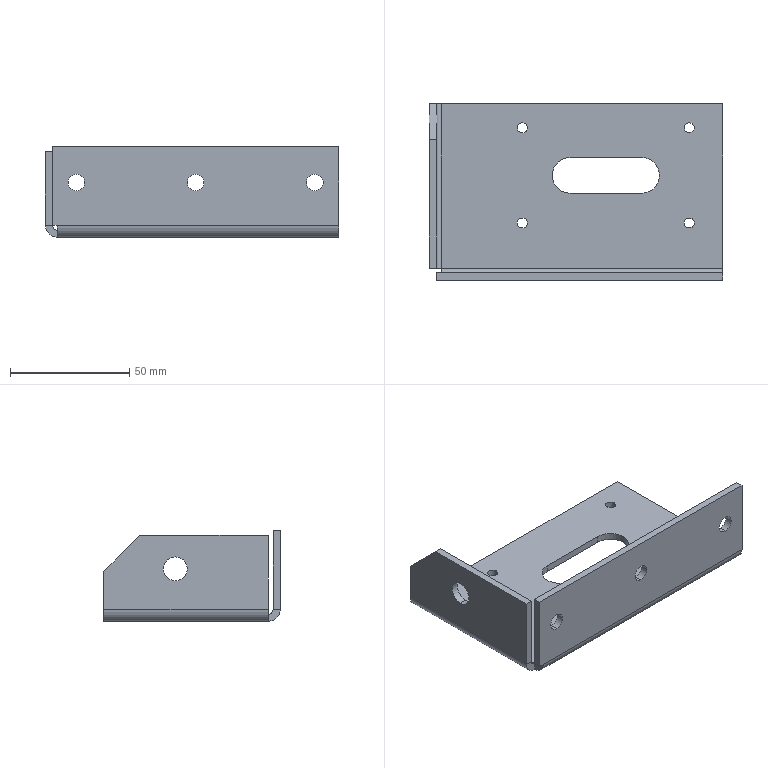Part | NX | features BREP 1 | 1 solid | 45 faces | box 123 x 74 x 38 mm | volume 42841 mm3 | cylinder 23 | plane 22 | commonest cylinder face diameters 4.2 x8 7 x6 10 x4 15 x3 4 x2
STEP:
#1=CARTESIAN_POINT('',(-123.,59.,-2.));
#2=VERTEX_POINT('',#1);
#3=CARTESIAN_POINT('',(-123.,74.,-17.));
#4=VERTEX_POINT('',#3);
#5=CARTESIAN_POINT('',(-123.,28.5,28.5));
#6=DIRECTION('',(0.,0.7071,-0.7071));
#7=VECTOR('',#6,1000.);
#8=LINE('',#5,#7);
#9=EDGE_CURVE('',#2,#4,#8,.T.);
#10=ORIENTED_EDGE('',*,*,#9,.F.);
#11=CARTESIAN_POINT('',(-120.,59.,-2.));
#12=VERTEX_POINT('',#11);
#13=CARTESIAN_POINT('',(-123.,59.,-2.));
#14=DIRECTION('',(-1.,0.,0.));
#15=VECTOR('',#14,1000.);
#16=LINE('',#13,#15);
#17=EDGE_CURVE('',#12,#2,#16,.T.);
#18=ORIENTED_EDGE('',*,*,#17,.F.);
#19=CARTESIAN_POINT('',(-120.,74.,-17.));
#20=VERTEX_POINT('',#19);
#21=CARTESIAN_POINT('',(-120.,74.,-17.));
#22=DIRECTION('',(0.,-0.7071,0.7071));
#23=VECTOR('',#22,1000.);
#24=LINE('',#21,#23);
#25=EDGE_CURVE('',#20,#12,#24,.T.);
#26=ORIENTED_EDGE('',*,*,#25,.F.);
#27=CARTESIAN_POINT('',(-123.,74.,-17.));
#28=DIRECTION('',(1.,0.,0.));
#29=VECTOR('',#28,1000.);
#30=LINE('',#27,#29);
#31=EDGE_CURVE('',#4,#20,#30,.T.);
#32=ORIENTED_EDGE('',*,*,#31,.F.);
#33=EDGE_LOOP('',(#10,#18,#26,#32));
#34=FACE_BOUND('',#33,.T.);
#35=CARTESIAN_POINT('',(-123.,74.,-17.));
#36=DIRECTION('',(0.,-0.7071,-0.7071));
#37=DIRECTION('',(1.,0.,0.));
#38=AXIS2_PLACEMENT_3D('',#35,#36,#37);
#39=PLANE('',#38);
#40=ADVANCED_FACE('',(#34),#39,.F.);
#41=CARTESIAN_POINT('',(-110.,3.,-18.5));
#42=VERTEX_POINT('',#41);
#43=CARTESIAN_POINT('',(-110.,0.,-18.5));
#44=VERTEX_POINT('',#43);
#45=CARTESIAN_POINT('',(-110.,3.,-18.5));
#46=DIRECTION('',(0.,1.,0.));
#47=VECTOR('',#46,1000.);
#48=LINE('',#45,#47);
#49=EDGE_CURVE('',#42,#44,#48,.F.);
#50=ORIENTED_EDGE('',*,*,#49,.T.);
#51=CARTESIAN_POINT('',(-110.,0.,-11.5));
#52=VERTEX_POINT('',#51);
#53=CARTESIAN_POINT('',(-110.,0.,-15.));
#54=DIRECTION('',(0.,1.,0.));
#55=DIRECTION('',(0.,0.,1.));
#56=AXIS2_PLACEMENT_3D('',#53,#54,#55);
#57=CIRCLE('',#56,3.5);
#58=EDGE_CURVE('',#52,#44,#57,.T.);
#59=ORIENTED_EDGE('',*,*,#58,.F.);
#60=CARTESIAN_POINT('',(-110.,3.,-11.5));
#61=VERTEX_POINT('',#60);
#62=CARTESIAN_POINT('',(-110.,3.,-11.5));
#63=DIRECTION('',(0.,1.,0.));
#64=VECTOR('',#63,1000.);
#65=LINE('',#62,#64);
#66=EDGE_CURVE('',#61,#52,#65,.F.);
#67=ORIENTED_EDGE('',*,*,#66,.F.);
#68=CARTESIAN_POINT('',(-110.,3.,-15.));
#69=DIRECTION('',(0.,1.,0.));
#70=DIRECTION('',(0.,0.,1.));
#71=AXIS2_PLACEMENT_3D('',#68,#69,#70);
#72=CIRCLE('',#71,3.5);
#73=EDGE_CURVE('',#61,#42,#72,.T.);
#74=ORIENTED_EDGE('',*,*,#73,.T.);
#75=EDGE_LOOP('',(#50,#59,#67,#74));
#76=FACE_BOUND('',#75,.T.);
#77=CARTESIAN_POINT('',(-110.,3.,-15.));
#78=DIRECTION('',(0.,1.,0.));
#79=DIRECTION('',(0.,0.,1.));
#80=AXIS2_PLACEMENT_3D('',#77,#78,#79);
#81=CYLINDRICAL_SURFACE('',#80,3.5);
#82=ADVANCED_FACE('',(#76),#81,.F.);
#83=CARTESIAN_POINT('',(-60.,3.,-18.5));
#84=VERTEX_POINT('',#83);
#85=CARTESIAN_POINT('',(-60.,0.,-18.5));
#86=VERTEX_POINT('',#85);
#87=CARTESIAN_POINT('',(-60.,3.,-18.5));
#88=DIRECTION('',(0.,1.,0.));
#89=VECTOR('',#88,1000.);
#90=LINE('',#87,#89);
#91=EDGE_CURVE('',#84,#86,#90,.F.);
#92=ORIENTED_EDGE('',*,*,#91,.T.);
#93=CARTESIAN_POINT('',(-60.,0.,-11.5));
#94=VERTEX_POINT('',#93);
#95=CARTESIAN_POINT('',(-60.,0.,-15.));
#96=DIRECTION('',(0.,1.,0.));
#97=DIRECTION('',(0.,0.,1.));
#98=AXIS2_PLACEMENT_3D('',#95,#96,#97);
#99=CIRCLE('',#98,3.5);
#100=EDGE_CURVE('',#94,#86,#99,.T.);
#101=ORIENTED_EDGE('',*,*,#100,.F.);
#102=CARTESIAN_POINT('',(-60.,3.,-11.5));
#103=VERTEX_POINT('',#102);
#104=CARTESIAN_POINT('',(-60.,3.,-11.5));
#105=DIRECTION('',(0.,1.,0.));
#106=VECTOR('',#105,1000.);
#107=LINE('',#104,#106);
#108=EDGE_CURVE('',#103,#94,#107,.F.);
#109=ORIENTED_EDGE('',*,*,#108,.F.);
#110=CARTESIAN_POINT('',(-60.,3.,-15.));
#111=DIRECTION('',(0.,1.,0.));
#112=DIRECTION('',(0.,0.,1.));
#113=AXIS2_PLACEMENT_3D('',#110,#111,#112);
#114=CIRCLE('',#113,3.5);
#115=EDGE_CURVE('',#103,#84,#114,.T.);
#116=ORIENTED_EDGE('',*,*,#115,.T.);
#117=EDGE_LOOP('',(#92,#101,#109,#116));
#118=FACE_BOUND('',#117,.T.);
#119=CARTESIAN_POINT('',(-60.,3.,-15.));
#120=DIRECTION('',(0.,1.,0.));
#121=DIRECTION('',(0.,0.,1.));
#122=AXIS2_PLACEMENT_3D('',#119,#120,#121);
#123=CYLINDRICAL_SURFACE('',#122,3.5);
#124=ADVANCED_FACE('',(#118),#123,.F.);
#125=CARTESIAN_POINT('',(-10.,3.,-18.5));
#126=VERTEX_POINT('',#125);
#127=CARTESIAN_POINT('',(-10.,0.,-18.5));
#128=VERTEX_POINT('',#127);
#129=CARTESIAN_POINT('',(-10.,3.,-18.5));
#130=DIRECTION('',(0.,1.,0.));
#131=VECTOR('',#130,1000.);
#132=LINE('',#129,#131);
#133=EDGE_CURVE('',#126,#128,#132,.F.);
#134=ORIENTED_EDGE('',*,*,#133,.T.);
#135=CARTESIAN_POINT('',(-10.,0.,-11.5));
#136=VERTEX_POINT('',#135);
#137=CARTESIAN_POINT('',(-10.,0.,-15.));
#138=DIRECTION('',(0.,1.,0.));
#139=DIRECTION('',(0.,0.,1.));
#140=AXIS2_PLACEMENT_3D('',#137,#138,#139);
#141=CIRCLE('',#140,3.5);
#142=EDGE_CURVE('',#136,#128,#141,.T.);
#143=ORIENTED_EDGE('',*,*,#142,.F.);
#144=CARTESIAN_POINT('',(-10.,3.,-11.5));
#145=VERTEX_POINT('',#144);
#146=CARTESIAN_POINT('',(-10.,3.,-11.5));
#147=DIRECTION('',(0.,1.,0.));
#148=VECTOR('',#147,1000.);
#149=LINE('',#146,#148);
#150=EDGE_CURVE('',#145,#136,#149,.F.);
#151=ORIENTED_EDGE('',*,*,#150,.F.);
#152=CARTESIAN_POINT('',(-10.,3.,-15.));
#153=DIRECTION('',(0.,1.,0.));
#154=DIRECTION('',(0.,0.,1.));
#155=AXIS2_PLACEMENT_3D('',#152,#153,#154);
#156=CIRCLE('',#155,3.5);
#157=EDGE_CURVE('',#145,#126,#156,.T.);
#158=ORIENTED_EDGE('',*,*,#157,.T.);
#159=EDGE_LOOP('',(#134,#143,#151,#158));
#160=FACE_BOUND('',#159,.T.);
#161=CARTESIAN_POINT('',(-10.,3.,-15.));
#162=DIRECTION('',(0.,1.,0.));
#163=DIRECTION('',(0.,0.,1.));
#164=AXIS2_PLACEMENT_3D('',#161,#162,#163);
#165=CYLINDRICAL_SURFACE('',#164,3.5);
#166=ADVANCED_FACE('',(#160),#165,.F.);
#167=CARTESIAN_POINT('',(-86.1,64.,-35.));
#168=VERTEX_POINT('',#167);
#169=CARTESIAN_POINT('',(-86.1,64.,-38.));
#170=VERTEX_POINT('',#169);
#171=CARTESIAN_POINT('',(-86.1,64.,-35.));
#172=DIRECTION('',(0.,0.,1.));
#173=VECTOR('',#172,1000.);
#174=LINE('',#171,#173);
#175=EDGE_CURVE('',#168,#170,#174,.F.);
#176=ORIENTED_EDGE('',*,*,#175,.T.);
#177=CARTESIAN_POINT('',(-81.9,64.,-38.));
#178=VERTEX_POINT('',#177);
#179=CARTESIAN_POINT('',(-84.,64.,-38.));
#180=DIRECTION('',(0.,0.,1.));
#181=DIRECTION('',(1.,0.,0.));
#182=AXIS2_PLACEMENT_3D('',#179,#180,#181);
#183=CIRCLE('',#182,2.1);
#184=EDGE_CURVE('',#178,#170,#183,.T.);
#185=ORIENTED_EDGE('',*,*,#184,.F.);
#186=CARTESIAN_POINT('',(-81.9,64.,-35.));
#187=VERTEX_POINT('',#186);
#188=CARTESIAN_POINT('',(-81.9,64.,-35.));
#189=DIRECTION('',(0.,0.,1.));
#190=VECTOR('',#189,1000.);
#191=LINE('',#188,#190);
#192=EDGE_CURVE('',#187,#178,#191,.F.);
#193=ORIENTED_EDGE('',*,*,#192,.F.);
#194=CARTESIAN_POINT('',(-84.,64.,-35.));
#195=DIRECTION('',(0.,0.,1.));
#196=DIRECTION('',(1.,0.,0.));
#197=AXIS2_PLACEMENT_3D('',#194,#195,#196);
#198=CIRCLE('',#197,2.1);
#199=EDGE_CURVE('',#187,#168,#198,.T.);
#200=ORIENTED_EDGE('',*,*,#199,.T.);
#201=EDGE_LOOP('',(#176,#185,#193,#200));
#202=FACE_BOUND('',#201,.T.);
#203=CARTESIAN_POINT('',(-84.,64.,-35.));
#204=DIRECTION('',(0.,0.,1.));
#205=DIRECTION('',(1.,0.,0.));
#206=AXIS2_PLACEMENT_3D('',#203,#204,#205);
#207=CYLINDRICAL_SURFACE('',#206,2.1);
#208=ADVANCED_FACE('',(#202),#207,.F.);
#209=CARTESIAN_POINT('',(-86.1,24.,-35.));
#210=VERTEX_POINT('',#209);
#211=CARTESIAN_POINT('',(-86.1,24.,-38.));
#212=VERTEX_POINT('',#211);
#213=CARTESIAN_POINT('',(-86.1,24.,-35.));
#214=DIRECTION('',(0.,0.,1.));
#215=VECTOR('',#214,1000.);
#216=LINE('',#213,#215);
#217=EDGE_CURVE('',#210,#212,#216,.F.);
#218=ORIENTED_EDGE('',*,*,#217,.T.);
#219=CARTESIAN_POINT('',(-81.9,24.,-38.));
#220=VERTEX_POINT('',#219);
#221=CARTESIAN_POINT('',(-84.,24.,-38.));
#222=DIRECTION('',(0.,0.,1.));
#223=DIRECTION('',(1.,0.,0.));
#224=AXIS2_PLACEMENT_3D('',#221,#222,#223);
#225=CIRCLE('',#224,2.1);
#226=EDGE_CURVE('',#220,#212,#225,.T.);
#227=ORIENTED_EDGE('',*,*,#226,.F.);
#228=CARTESIAN_POINT('',(-81.9,24.,-35.));
#229=VERTEX_POINT('',#228);
#230=CARTESIAN_POINT('',(-81.9,24.,-35.));
#231=DIRECTION('',(0.,0.,1.));
#232=VECTOR('',#231,1000.);
#233=LINE('',#230,#232);
#234=EDGE_CURVE('',#229,#220,#233,.F.);
#235=ORIENTED_EDGE('',*,*,#234,.F.);
#236=CARTESIAN_POINT('',(-84.,24.,-35.));
#237=DIRECTION('',(0.,0.,1.));
#238=DIRECTION('',(1.,0.,0.));
#239=AXIS2_PLACEMENT_3D('',#236,#237,#238);
#240=CIRCLE('',#239,2.1);
#241=EDGE_CURVE('',#229,#210,#240,.T.);
#242=ORIENTED_EDGE('',*,*,#241,.T.);
#243=EDGE_LOOP('',(#218,#227,#235,#242));
#244=FACE_BOUND('',#243,.T.);
#245=CARTESIAN_POINT('',(-84.,24.,-35.));
#246=DIRECTION('',(0.,0.,1.));
#247=DIRECTION('',(1.,0.,0.));
#248=AXIS2_PLACEMENT_3D('',#245,#246,#247);
#249=CYLINDRICAL_SURFACE('',#248,2.1);
#250=ADVANCED_FACE('',(#244),#249,.F.);
#251=CARTESIAN_POINT('',(-16.1,24.,-35.));
#252=VERTEX_POINT('',#251);
#253=CARTESIAN_POINT('',(-16.1,24.,-38.));
#254=VERTEX_POINT('',#253);
#255=CARTESIAN_POINT('',(-16.1,24.,-35.));
#256=DIRECTION('',(0.,0.,1.));
#257=VECTOR('',#256,1000.);
#258=LINE('',#255,#257);
#259=EDGE_CURVE('',#252,#254,#258,.F.);
#260=ORIENTED_EDGE('',*,*,#259,.T.);
#261=CARTESIAN_POINT('',(-11.9,24.,-38.));
#262=VERTEX_POINT('',#261);
#263=CARTESIAN_POINT('',(-14.,24.,-38.));
#264=DIRECTION('',(0.,0.,1.));
#265=DIRECTION('',(1.,0.,0.));
#266=AXIS2_PLACEMENT_3D('',#263,#264,#265);
#267=CIRCLE('',#266,2.1);
#268=EDGE_CURVE('',#262,#254,#267,.T.);
#269=ORIENTED_EDGE('',*,*,#268,.F.);
#270=CARTESIAN_POINT('',(-11.9,24.,-35.));
#271=VERTEX_POINT('',#270);
#272=CARTESIAN_POINT('',(-11.9,24.,-35.));
#273=DIRECTION('',(0.,0.,1.));
#274=VECTOR('',#273,1000.);
#275=LINE('',#272,#274);
#276=EDGE_CURVE('',#271,#262,#275,.F.);
#277=ORIENTED_EDGE('',*,*,#276,.F.);
#278=CARTESIAN_POINT('',(-14.,24.,-35.));
#279=DIRECTION('',(0.,0.,1.));
#280=DIRECTION('',(1.,0.,0.));
#281=AXIS2_PLACEMENT_3D('',#278,#279,#280);
#282=CIRCLE('',#281,2.1);
#283=EDGE_CURVE('',#271,#252,#282,.T.);
#284=ORIENTED_EDGE('',*,*,#283,.T.);
#285=EDGE_LOOP('',(#260,#269,#277,#284));
#286=FACE_BOUND('',#285,.T.);
#287=CARTESIAN_POINT('',(-14.,24.,-35.));
#288=DIRECTION('',(0.,0.,1.));
#289=DIRECTION('',(1.,0.,0.));
#290=AXIS2_PLACEMENT_3D('',#287,#288,#289);
#291=CYLINDRICAL_SURFACE('',#290,2.1);
#292=ADVANCED_FACE('',(#286),#291,.F.);
#293=CARTESIAN_POINT('',(-16.1,64.,-35.));
#294=VERTEX_POINT('',#293);
#295=CARTESIAN_POINT('',(-16.1,64.,-38.));
#296=VERTEX_POINT('',#295);
#297=CARTESIAN_POINT('',(-16.1,64.,-35.));
#298=DIRECTION('',(0.,0.,1.));
#299=VECTOR('',#298,1000.);
#300=LINE('',#297,#299);
#301=EDGE_CURVE('',#294,#296,#300,.F.);
#302=ORIENTED_EDGE('',*,*,#301,.T.);
#303=CARTESIAN_POINT('',(-11.9,64.,-38.));
#304=VERTEX_POINT('',#303);
#305=CARTESIAN_POINT('',(-14.,64.,-38.));
#306=DIRECTION('',(0.,0.,1.));
#307=DIRECTION('',(1.,0.,0.));
#308=AXIS2_PLACEMENT_3D('',#305,#306,#307);
#309=CIRCLE('',#308,2.1);
#310=EDGE_CURVE('',#304,#296,#309,.T.);
#311=ORIENTED_EDGE('',*,*,#310,.F.);
#312=CARTESIAN_POINT('',(-11.9,64.,-35.));
#313=VERTEX_POINT('',#312);
#314=CARTESIAN_POINT('',(-11.9,64.,-35.));
#315=DIRECTION('',(0.,0.,1.));
#316=VECTOR('',#315,1000.);
#317=LINE('',#314,#316);
#318=EDGE_CURVE('',#313,#304,#317,.F.);
#319=ORIENTED_EDGE('',*,*,#318,.F.);
#320=CARTESIAN_POINT('',(-14.,64.,-35.));
#321=DIRECTION('',(0.,0.,1.));
#322=DIRECTION('',(1.,0.,0.));
#323=AXIS2_PLACEMENT_3D('',#320,#321,#322);
#324=CIRCLE('',#323,2.1);
#325=EDGE_CURVE('',#313,#294,#324,.T.);
#326=ORIENTED_EDGE('',*,*,#325,.T.);
#327=EDGE_LOOP('',(#302,#311,#319,#326));
#328=FACE_BOUND('',#327,.T.);
#329=CARTESIAN_POINT('',(-14.,64.,-35.));
#330=DIRECTION('',(0.,0.,1.));
#331=DIRECTION('',(1.,0.,0.));
#332=AXIS2_PLACEMENT_3D('',#329,#330,#331);
#333=CYLINDRICAL_SURFACE('',#332,2.1);
#334=ADVANCED_FACE('',(#328),#333,.F.);
#335=CARTESIAN_POINT('',(-34.,51.5,-35.));
#336=VERTEX_POINT('',#335);
#337=CARTESIAN_POINT('',(-64.,51.5,-35.));
#338=VERTEX_POINT('',#337);
#339=CARTESIAN_POINT('',(-34.,51.5,-35.));
#340=DIRECTION('',(-1.,0.,0.));
#341=VECTOR('',#340,1000.);
#342=LINE('',#339,#341);
#343=EDGE_CURVE('',#336,#338,#342,.T.);
#344=ORIENTED_EDGE('',*,*,#343,.T.);
#345=CARTESIAN_POINT('',(-64.,51.5,-38.));
#346=VERTEX_POINT('',#345);
#347=CARTESIAN_POINT('',(-64.,51.5,-38.));
#348=DIRECTION('',(0.,0.,1.));
#349=VECTOR('',#348,1000.);
#350=LINE('',#347,#349);
#351=EDGE_CURVE('',#346,#338,#350,.T.);
#352=ORIENTED_EDGE('',*,*,#351,.F.);
#353=CARTESIAN_POINT('',(-34.,51.5,-38.));
#354=VERTEX_POINT('',#353);
#355=CARTESIAN_POINT('',(-34.,51.5,-38.));
#356=DIRECTION('',(-1.,0.,0.));
#357=VECTOR('',#356,1000.);
#358=LINE('',#355,#357);
#359=EDGE_CURVE('',#354,#346,#358,.T.);
#360=ORIENTED_EDGE('',*,*,#359,.F.);
#361=CARTESIAN_POINT('',(-34.,51.5,-38.));
#362=DIRECTION('',(0.,0.,1.));
#363=VECTOR('',#362,1000.);
#364=LINE('',#361,#363);
#365=EDGE_CURVE('',#354,#336,#364,.T.);
#366=ORIENTED_EDGE('',*,*,#365,.T.);
#367=EDGE_LOOP('',(#344,#352,#360,#366));
#368=FACE_BOUND('',#367,.T.);
#369=CARTESIAN_POINT('',(-34.,51.5,-38.));
#370=DIRECTION('',(0.,1.,0.));
#371=DIRECTION('',(0.,0.,1.));
#372=AXIS2_PLACEMENT_3D('',#369,#370,#371);
#373=PLANE('',#372);
#374=ADVANCED_FACE('',(#368),#373,.F.);
#375=CARTESIAN_POINT('',(-64.,36.5,-35.));
#376=VERTEX_POINT('',#375);
#377=CARTESIAN_POINT('',(-64.,44.,-35.));
#378=DIRECTION('',(0.,0.,1.));
#379=DIRECTION('',(1.,0.,0.));
#380=AXIS2_PLACEMENT_3D('',#377,#378,#379);
#381=CIRCLE('',#380,7.5);
#382=EDGE_CURVE('',#338,#376,#381,.T.);
#383=ORIENTED_EDGE('',*,*,#382,.T.);
#384=CARTESIAN_POINT('',(-64.,36.5,-38.));
#385=VERTEX_POINT('',#384);
#386=CARTESIAN_POINT('',(-64.,36.5,-38.));
#387=DIRECTION('',(0.,0.,1.));
#388=VECTOR('',#387,1000.);
#389=LINE('',#386,#388);
#390=EDGE_CURVE('',#385,#376,#389,.T.);
#391=ORIENTED_EDGE('',*,*,#390,.F.);
#392=CARTESIAN_POINT('',(-64.,44.,-38.));
#393=DIRECTION('',(0.,0.,1.));
#394=DIRECTION('',(1.,0.,0.));
#395=AXIS2_PLACEMENT_3D('',#392,#393,#394);
#396=CIRCLE('',#395,7.5);
#397=EDGE_CURVE('',#346,#385,#396,.T.);
#398=ORIENTED_EDGE('',*,*,#397,.F.);
#399=ORIENTED_EDGE('',*,*,#351,.T.);
#400=EDGE_LOOP('',(#383,#391,#398,#399));
#401=FACE_BOUND('',#400,.T.);
#402=CARTESIAN_POINT('',(-64.,44.,-38.));
#403=DIRECTION('',(0.,0.,1.));
#404=DIRECTION('',(1.,0.,0.));
#405=AXIS2_PLACEMENT_3D('',#402,#403,#404);
#406=CYLINDRICAL_SURFACE('',#405,7.5);
#407=ADVANCED_FACE('',(#401),#406,.F.);
#408=CARTESIAN_POINT('',(-34.,36.5,-35.));
#409=VERTEX_POINT('',#408);
#410=CARTESIAN_POINT('',(-34.,36.5,-35.));
#411=DIRECTION('',(1.,0.,0.));
#412=VECTOR('',#411,1000.);
#413=LINE('',#410,#412);
#414=EDGE_CURVE('',#376,#409,#413,.T.);
#415=ORIENTED_EDGE('',*,*,#414,.T.);
#416=CARTESIAN_POINT('',(-34.,36.5,-38.));
#417=VERTEX_POINT('',#416);
#418=CARTESIAN_POINT('',(-34.,36.5,-38.));
#419=DIRECTION('',(0.,0.,1.));
#420=VECTOR('',#419,1000.);
#421=LINE('',#418,#420);
#422=EDGE_CURVE('',#417,#409,#421,.T.);
#423=ORIENTED_EDGE('',*,*,#422,.F.);
#424=CARTESIAN_POINT('',(-34.,36.5,-38.));
#425=DIRECTION('',(1.,0.,0.));
#426=VECTOR('',#425,1000.);
#427=LINE('',#424,#426);
#428=EDGE_CURVE('',#385,#417,#427,.T.);
#429=ORIENTED_EDGE('',*,*,#428,.F.);
#430=ORIENTED_EDGE('',*,*,#390,.T.);
#431=EDGE_LOOP('',(#415,#423,#429,#430));
#432=FACE_BOUND('',#431,.T.);
#433=CARTESIAN_POINT('',(-34.,36.5,-38.));
#434=DIRECTION('',(0.,-1.,0.));
#435=DIRECTION('',(1.,0.,0.));
#436=AXIS2_PLACEMENT_3D('',#433,#434,#435);
#437=PLANE('',#436);
#438=ADVANCED_FACE('',(#432),#437,.F.);
#439=CARTESIAN_POINT('',(-26.5,44.,-38.));
#440=VERTEX_POINT('',#439);
#441=CARTESIAN_POINT('',(-26.5,44.,-35.));
#442=VERTEX_POINT('',#441);
#443=CARTESIAN_POINT('',(-26.5,44.,-38.));
#444=DIRECTION('',(0.,0.,1.));
#445=VECTOR('',#444,1000.);
#446=LINE('',#443,#445);
#447=EDGE_CURVE('',#440,#442,#446,.T.);
#448=ORIENTED_EDGE('',*,*,#447,.F.);
#449=CARTESIAN_POINT('',(-34.,44.,-38.));
#450=DIRECTION('',(0.,0.,1.));
#451=DIRECTION('',(1.,0.,0.));
#452=AXIS2_PLACEMENT_3D('',#449,#450,#451);
#453=CIRCLE('',#452,7.5);
#454=EDGE_CURVE('',#417,#440,#453,.T.);
#455=ORIENTED_EDGE('',*,*,#454,.F.);
#456=ORIENTED_EDGE('',*,*,#422,.T.);
#457=CARTESIAN_POINT('',(-34.,44.,-35.));
#458=DIRECTION('',(0.,0.,1.));
#459=DIRECTION('',(1.,0.,0.));
#460=AXIS2_PLACEMENT_3D('',#457,#458,#459);
#461=CIRCLE('',#460,7.5);
#462=EDGE_CURVE('',#409,#442,#461,.T.);
#463=ORIENTED_EDGE('',*,*,#462,.T.);
#464=EDGE_LOOP('',(#448,#455,#456,#463));
#465=FACE_BOUND('',#464,.T.);
#466=CARTESIAN_POINT('',(-34.,44.,-38.));
#467=DIRECTION('',(0.,0.,1.));
#468=DIRECTION('',(1.,0.,0.));
#469=AXIS2_PLACEMENT_3D('',#466,#467,#468);
#470=CYLINDRICAL_SURFACE('',#469,7.5);
#471=ADVANCED_FACE('',(#465),#470,.F.);
#472=CARTESIAN_POINT('',(-123.,44.,-21.));
#473=VERTEX_POINT('',#472);
#474=CARTESIAN_POINT('',(-120.,44.,-21.));
#475=VERTEX_POINT('',#474);
#476=CARTESIAN_POINT('',(-123.,44.,-21.));
#477=DIRECTION('',(-1.,0.,0.));
#478=VECTOR('',#477,1000.);
#479=LINE('',#476,#478);
#480=EDGE_CURVE('',#473,#475,#479,.F.);
#481=ORIENTED_EDGE('',*,*,#480,.T.);
#482=CARTESIAN_POINT('',(-120.,44.,-11.));
#483=VERTEX_POINT('',#482);
#484=CARTESIAN_POINT('',(-120.,44.,-16.));
#485=DIRECTION('',(-1.,0.,0.));
#486=DIRECTION('',(0.,0.,1.));
#487=AXIS2_PLACEMENT_3D('',#484,#485,#486);
#488=CIRCLE('',#487,5.);
#489=EDGE_CURVE('',#483,#475,#488,.T.);
#490=ORIENTED_EDGE('',*,*,#489,.F.);
#491=CARTESIAN_POINT('',(-123.,44.,-11.));
#492=VERTEX_POINT('',#491);
#493=CARTESIAN_POINT('',(-123.,44.,-11.));
#494=DIRECTION('',(-1.,0.,0.));
#495=VECTOR('',#494,1000.);
#496=LINE('',#493,#495);
#497=EDGE_CURVE('',#492,#483,#496,.F.);
#498=ORIENTED_EDGE('',*,*,#497,.F.);
#499=CARTESIAN_POINT('',(-123.,44.,-16.));
#500=DIRECTION('',(-1.,0.,0.));
#501=DIRECTION('',(0.,0.,1.));
#502=AXIS2_PLACEMENT_3D('',#499,#500,#501);
#503=CIRCLE('',#502,5.);
#504=EDGE_CURVE('',#492,#473,#503,.T.);
#505=ORIENTED_EDGE('',*,*,#504,.T.);
#506=EDGE_LOOP('',(#481,#490,#498,#505));
#507=FACE_BOUND('',#506,.T.);
#508=CARTESIAN_POINT('',(-123.,44.,-16.));
#509=DIRECTION('',(-1.,0.,0.));
#510=DIRECTION('',(0.,0.,1.));
#511=AXIS2_PLACEMENT_3D('',#508,#509,#510);
#512=CYLINDRICAL_SURFACE('',#511,5.);
#513=ADVANCED_FACE('',(#507),#512,.F.);
#514=CARTESIAN_POINT('',(-120.,5.,-2.));
#515=VERTEX_POINT('',#514);
#516=CARTESIAN_POINT('',(-120.,5.,-2.));
#517=DIRECTION('',(0.,-1.,0.));
#518=VECTOR('',#517,1000.);
#519=LINE('',#516,#518);
#520=EDGE_CURVE('',#12,#515,#519,.T.);
#521=ORIENTED_EDGE('',*,*,#520,.F.);
#522=ORIENTED_EDGE('',*,*,#17,.T.);
#523=CARTESIAN_POINT('',(-123.,5.,-2.));
#524=VERTEX_POINT('',#523);
#525=CARTESIAN_POINT('',(-123.,5.,-2.));
#526=DIRECTION('',(0.,-1.,0.));
#527=VECTOR('',#526,1000.);
#528=LINE('',#525,#527);
#529=EDGE_CURVE('',#2,#524,#528,.T.);
#530=ORIENTED_EDGE('',*,*,#529,.T.);
#531=CARTESIAN_POINT('',(-123.,5.,-2.));
#532=DIRECTION('',(1.,0.,0.));
#533=VECTOR('',#532,1000.);
#534=LINE('',#531,#533);
#535=EDGE_CURVE('',#524,#515,#534,.T.);
#536=ORIENTED_EDGE('',*,*,#535,.T.);
#537=EDGE_LOOP('',(#521,#522,#530,#536));
#538=FACE_BOUND('',#537,.T.);
#539=CARTESIAN_POINT('',(-123.,5.,-2.));
#540=DIRECTION('',(0.,0.,1.));
#541=DIRECTION('',(1.,0.,0.));
#542=AXIS2_PLACEMENT_3D('',#539,#540,#541);
#543=PLANE('',#542);
#544=ADVANCED_FACE('',(#538),#543,.T.);
#545=CARTESIAN_POINT('',(-120.,74.,-33.));
#546=VERTEX_POINT('',#545);
#547=CARTESIAN_POINT('',(-120.,74.,-2.));
#548=DIRECTION('',(0.,0.,1.));
#549=VECTOR('',#548,1000.);
#550=LINE('',#547,#549);
#551=EDGE_CURVE('',#546,#20,#550,.T.);
#552=ORIENTED_EDGE('',*,*,#551,.T.);
#553=ORIENTED_EDGE('',*,*,#25,.T.);
#554=ORIENTED_EDGE('',*,*,#520,.T.);
#555=CARTESIAN_POINT('',(-120.,5.,-33.));
#556=VERTEX_POINT('',#555);
#557=CARTESIAN_POINT('',(-120.,5.,-35.));
#558=DIRECTION('',(0.,0.,-1.));
#559=VECTOR('',#558,1000.);
#560=LINE('',#557,#559);
#561=EDGE_CURVE('',#515,#556,#560,.T.);
#562=ORIENTED_EDGE('',*,*,#561,.T.);
#563=CARTESIAN_POINT('',(-120.,74.,-33.));
#564=DIRECTION('',(0.,-1.,0.));
#565=VECTOR('',#564,1000.);
#566=LINE('',#563,#565);
#567=EDGE_CURVE('',#546,#556,#566,.T.);
#568=ORIENTED_EDGE('',*,*,#567,.F.);
#569=EDGE_LOOP('',(#552,#553,#554,#562,#568));
#570=FACE_BOUND('',#569,.T.);
#571=ORIENTED_EDGE('',*,*,#489,.T.);
#572=CARTESIAN_POINT('',(-120.,44.,-16.));
#573=DIRECTION('',(-1.,0.,0.));
#574=DIRECTION('',(0.,0.,1.));
#575=AXIS2_PLACEMENT_3D('',#572,#573,#574);
#576=CIRCLE('',#575,5.);
#577=EDGE_CURVE('',#475,#483,#576,.T.);
#578=ORIENTED_EDGE('',*,*,#577,.T.);
#579=EDGE_LOOP('',(#571,#578));
#580=FACE_BOUND('',#579,.T.);
#581=CARTESIAN_POINT('',(-120.,0.,0.));
#582=DIRECTION('',(-1.,0.,0.));
#583=DIRECTION('',(0.,0.,1.));
#584=AXIS2_PLACEMENT_3D('',#581,#582,#583);
#585=PLANE('',#584);
#586=ADVANCED_FACE('',(#570,#580),#585,.F.);
#587=ORIENTED_EDGE('',*,*,#529,.F.);
#588=ORIENTED_EDGE('',*,*,#9,.T.);
#589=CARTESIAN_POINT('',(-123.,74.,-33.));
#590=VERTEX_POINT('',#589);
#591=CARTESIAN_POINT('',(-123.,74.,-2.));
#592=DIRECTION('',(0.,0.,1.));
#593=VECTOR('',#592,1000.);
#594=LINE('',#591,#593);
#595=EDGE_CURVE('',#590,#4,#594,.T.);
#596=ORIENTED_EDGE('',*,*,#595,.F.);
#597=CARTESIAN_POINT('',(-123.,5.,-33.));
#598=VERTEX_POINT('',#597);
#599=CARTESIAN_POINT('',(-123.,0.,-33.));
#600=DIRECTION('',(0.,-1.,0.));
#601=VECTOR('',#600,1000.);
#602=LINE('',#599,#601);
#603=EDGE_CURVE('',#590,#598,#602,.T.);
#604=ORIENTED_EDGE('',*,*,#603,.T.);
#605=CARTESIAN_POINT('',(-123.,5.,-35.));
#606=DIRECTION('',(0.,0.,-1.));
#607=VECTOR('',#606,1000.);
#608=LINE('',#605,#607);
#609=EDGE_CURVE('',#524,#598,#608,.T.);
#610=ORIENTED_EDGE('',*,*,#609,.F.);
#611=EDGE_LOOP('',(#587,#588,#596,#604,#610));
#612=FACE_BOUND('',#611,.T.);
#613=ORIENTED_EDGE('',*,*,#504,.F.);
#614=CARTESIAN_POINT('',(-123.,44.,-16.));
#615=DIRECTION('',(-1.,0.,0.));
#616=DIRECTION('',(0.,0.,1.));
#617=AXIS2_PLACEMENT_3D('',#614,#615,#616);
#618=CIRCLE('',#617,5.);
#619=EDGE_CURVE('',#473,#492,#618,.T.);
#620=ORIENTED_EDGE('',*,*,#619,.F.);
#621=EDGE_LOOP('',(#613,#620));
#622=FACE_BOUND('',#621,.T.);
#623=CARTESIAN_POINT('',(-123.,0.,0.));
#624=DIRECTION('',(-1.,0.,0.));
#625=DIRECTION('',(0.,0.,1.));
#626=AXIS2_PLACEMENT_3D('',#623,#624,#625);
#627=PLANE('',#626);
#628=ADVANCED_FACE('',(#612,#622),#627,.T.);
#629=ORIENTED_EDGE('',*,*,#595,.T.);
#630=ORIENTED_EDGE('',*,*,#31,.T.);
#631=ORIENTED_EDGE('',*,*,#551,.F.);
#632=CARTESIAN_POINT('',(-120.,74.,-33.));
#633=DIRECTION('',(-1.,0.,0.));
#634=VECTOR('',#633,1000.);
#635=LINE('',#632,#634);
#636=EDGE_CURVE('',#546,#590,#635,.T.);
#637=ORIENTED_EDGE('',*,*,#636,.T.);
#638=EDGE_LOOP('',(#629,#630,#631,#637));
#639=FACE_BOUND('',#638,.T.);
#640=CARTESIAN_POINT('',(-123.,74.,-2.));
#641=DIRECTION('',(0.,1.,0.));
#642=DIRECTION('',(0.,0.,1.));
#643=AXIS2_PLACEMENT_3D('',#640,#641,#642);
#644=PLANE('',#643);
#645=ADVANCED_FACE('',(#639),#644,.T.);
#646=ORIENTED_EDGE('',*,*,#609,.T.);
#647=CARTESIAN_POINT('',(-120.,5.,-33.));
#648=DIRECTION('',(-1.,0.,0.));
#649=VECTOR('',#648,1000.);
#650=LINE('',#647,#649);
#651=EDGE_CURVE('',#556,#598,#650,.T.);
#652=ORIENTED_EDGE('',*,*,#651,.F.);
#653=ORIENTED_EDGE('',*,*,#561,.F.);
#654=ORIENTED_EDGE('',*,*,#535,.F.);
#655=EDGE_LOOP('',(#646,#652,#653,#654));
#656=FACE_BOUND('',#655,.T.);
#657=CARTESIAN_POINT('',(-123.,5.,-35.));
#658=DIRECTION('',(0.,-1.,0.));
#659=DIRECTION('',(0.,0.,-1.));
#660=AXIS2_PLACEMENT_3D('',#657,#658,#659);
#661=PLANE('',#660);
#662=ADVANCED_FACE('',(#656),#661,.T.);
#663=CARTESIAN_POINT('',(-118.,5.,-35.));
#664=VERTEX_POINT('',#663);
#665=CARTESIAN_POINT('',(-118.,74.,-35.));
#666=VERTEX_POINT('',#665);
#667=CARTESIAN_POINT('',(-118.,5.,-35.));
#668=DIRECTION('',(0.,1.,0.));
#669=VECTOR('',#668,1000.);
#670=LINE('',#667,#669);
#671=EDGE_CURVE('',#664,#666,#670,.T.);
#672=ORIENTED_EDGE('',*,*,#671,.T.);
#673=CARTESIAN_POINT('',(-118.,74.,-33.));
#674=DIRECTION('',(0.,1.,0.));
#675=DIRECTION('',(0.,0.,-1.));
#676=AXIS2_PLACEMENT_3D('',#673,#674,#675);
#677=CIRCLE('',#676,2.);
#678=EDGE_CURVE('',#666,#546,#677,.T.);
#679=ORIENTED_EDGE('',*,*,#678,.T.);
#680=ORIENTED_EDGE('',*,*,#567,.T.);
#681=CARTESIAN_POINT('',(-118.,5.,-33.));
#682=DIRECTION('',(0.,-1.,0.));
#683=DIRECTION('',(0.,0.,-1.));
#684=AXIS2_PLACEMENT_3D('',#681,#682,#683);
#685=CIRCLE('',#684,2.);
#686=EDGE_CURVE('',#556,#664,#685,.T.);
#687=ORIENTED_EDGE('',*,*,#686,.T.);
#688=EDGE_LOOP('',(#672,#679,#680,#687));
#689=FACE_BOUND('',#688,.T.);
#690=CARTESIAN_POINT('',(-118.,5.,-33.));
#691=DIRECTION('',(0.,-1.,0.));
#692=DIRECTION('',(-1.,0.,0.));
#693=AXIS2_PLACEMENT_3D('',#690,#691,#692);
#694=CYLINDRICAL_SURFACE('',#693,2.);
#695=ADVANCED_FACE('',(#689),#694,.F.);
#696=CARTESIAN_POINT('',(-118.,5.,-38.));
#697=VERTEX_POINT('',#696);
#698=CARTESIAN_POINT('',(-118.,74.,-38.));
#699=VERTEX_POINT('',#698);
#700=CARTESIAN_POINT('',(-118.,5.,-38.));
#701=DIRECTION('',(0.,1.,0.));
#702=VECTOR('',#701,1000.);
#703=LINE('',#700,#702);
#704=EDGE_CURVE('',#697,#699,#703,.T.);
#705=ORIENTED_EDGE('',*,*,#704,.F.);
#706=CARTESIAN_POINT('',(-118.,5.,-33.));
#707=DIRECTION('',(0.,-1.,0.));
#708=DIRECTION('',(0.,0.,-1.));
#709=AXIS2_PLACEMENT_3D('',#706,#707,#708);
#710=CIRCLE('',#709,5.);
#711=EDGE_CURVE('',#598,#697,#710,.T.);
#712=ORIENTED_EDGE('',*,*,#711,.F.);
#713=ORIENTED_EDGE('',*,*,#603,.F.);
#714=CARTESIAN_POINT('',(-118.,74.,-33.));
#715=DIRECTION('',(0.,1.,0.));
#716=DIRECTION('',(0.,0.,-1.));
#717=AXIS2_PLACEMENT_3D('',#714,#715,#716);
#718=CIRCLE('',#717,5.);
#719=EDGE_CURVE('',#699,#590,#718,.T.);
#720=ORIENTED_EDGE('',*,*,#719,.F.);
#721=EDGE_LOOP('',(#705,#712,#713,#720));
#722=FACE_BOUND('',#721,.T.);
#723=CARTESIAN_POINT('',(-118.,5.,-33.));
#724=DIRECTION('',(0.,-1.,0.));
#725=DIRECTION('',(-1.,0.,0.));
#726=AXIS2_PLACEMENT_3D('',#723,#724,#725);
#727=CYLINDRICAL_SURFACE('',#726,5.);
#728=ADVANCED_FACE('',(#722),#727,.T.);
#729=ORIENTED_EDGE('',*,*,#686,.F.);
#730=ORIENTED_EDGE('',*,*,#651,.T.);
#731=ORIENTED_EDGE('',*,*,#711,.T.);
#732=CARTESIAN_POINT('',(-118.,5.,-35.));
#733=DIRECTION('',(0.,0.,-1.));
#734=VECTOR('',#733,1000.);
#735=LINE('',#732,#734);
#736=EDGE_CURVE('',#664,#697,#735,.T.);
#737=ORIENTED_EDGE('',*,*,#736,.F.);
#738=EDGE_LOOP('',(#729,#730,#731,#737));
#739=FACE_BOUND('',#738,.T.);
#740=CARTESIAN_POINT('',(-118.,5.,-33.));
#741=DIRECTION('',(0.,1.,0.));
#742=DIRECTION('',(0.,0.,1.));
#743=AXIS2_PLACEMENT_3D('',#740,#741,#742);
#744=PLANE('',#743);
#745=ADVANCED_FACE('',(#739),#744,.F.);
#746=ORIENTED_EDGE('',*,*,#636,.F.);
#747=ORIENTED_EDGE('',*,*,#678,.F.);
#748=CARTESIAN_POINT('',(-118.,74.,-35.));
#749=DIRECTION('',(0.,0.,-1.));
#750=VECTOR('',#749,1000.);
#751=LINE('',#748,#750);
#752=EDGE_CURVE('',#666,#699,#751,.T.);
#753=ORIENTED_EDGE('',*,*,#752,.T.);
#754=ORIENTED_EDGE('',*,*,#719,.T.);
#755=EDGE_LOOP('',(#746,#747,#753,#754));
#756=FACE_BOUND('',#755,.T.);
#757=CARTESIAN_POINT('',(-118.,74.,-33.));
#758=DIRECTION('',(0.,1.,0.));
#759=DIRECTION('',(0.,0.,1.));
#760=AXIS2_PLACEMENT_3D('',#757,#758,#759);
#761=PLANE('',#760);
#762=ADVANCED_FACE('',(#756),#761,.T.);
#763=CARTESIAN_POINT('',(0.,5.,-38.));
#764=VERTEX_POINT('',#763);
#765=CARTESIAN_POINT('',(0.,74.,-38.));
#766=VERTEX_POINT('',#765);
#767=CARTESIAN_POINT('',(0.,0.,-38.));
#768=DIRECTION('',(0.,1.,0.));
#769=VECTOR('',#768,1000.);
#770=LINE('',#767,#769);
#771=EDGE_CURVE('',#764,#766,#770,.T.);
#772=ORIENTED_EDGE('',*,*,#771,.T.);
#773=CARTESIAN_POINT('',(0.,74.,-35.));
#774=VERTEX_POINT('',#773);
#775=CARTESIAN_POINT('',(0.,74.,-35.));
#776=DIRECTION('',(0.,0.,-1.));
#777=VECTOR('',#776,1000.);
#778=LINE('',#775,#777);
#779=EDGE_CURVE('',#774,#766,#778,.T.);
#780=ORIENTED_EDGE('',*,*,#779,.F.);
#781=CARTESIAN_POINT('',(0.,5.,-35.));
#782=VERTEX_POINT('',#781);
#783=CARTESIAN_POINT('',(0.,0.,-35.));
#784=DIRECTION('',(0.,1.,0.));
#785=VECTOR('',#784,1000.);
#786=LINE('',#783,#785);
#787=EDGE_CURVE('',#782,#774,#786,.T.);
#788=ORIENTED_EDGE('',*,*,#787,.F.);
#789=CARTESIAN_POINT('',(0.,5.,-35.));
#790=DIRECTION('',(0.,0.,-1.));
#791=VECTOR('',#790,1000.);
#792=LINE('',#789,#791);
#793=EDGE_CURVE('',#782,#764,#792,.T.);
#794=ORIENTED_EDGE('',*,*,#793,.T.);
#795=EDGE_LOOP('',(#772,#780,#788,#794));
#796=FACE_BOUND('',#795,.T.);
#797=CARTESIAN_POINT('',(0.,5.,-33.));
#798=DIRECTION('',(1.,0.,0.));
#799=DIRECTION('',(0.,0.,-1.));
#800=AXIS2_PLACEMENT_3D('',#797,#798,#799);
#801=PLANE('',#800);
#802=ADVANCED_FACE('',(#796),#801,.T.);
#803=CARTESIAN_POINT('',(-120.,3.,0.));
#804=VERTEX_POINT('',#803);
#805=CARTESIAN_POINT('',(-120.,3.,-33.));
#806=VERTEX_POINT('',#805);
#807=CARTESIAN_POINT('',(-120.,3.,0.));
#808=DIRECTION('',(0.,0.,-1.));
#809=VECTOR('',#808,1000.);
#810=LINE('',#807,#809);
#811=EDGE_CURVE('',#804,#806,#810,.T.);
#812=ORIENTED_EDGE('',*,*,#811,.T.);
#813=CARTESIAN_POINT('',(-120.,0.,-33.));
#814=VERTEX_POINT('',#813);
#815=CARTESIAN_POINT('',(-120.,3.,-33.));
#816=DIRECTION('',(0.,-1.,0.));
#817=VECTOR('',#816,1000.);
#818=LINE('',#815,#817);
#819=EDGE_CURVE('',#806,#814,#818,.T.);
#820=ORIENTED_EDGE('',*,*,#819,.T.);
#821=CARTESIAN_POINT('',(-120.,0.,0.));
#822=VERTEX_POINT('',#821);
#823=CARTESIAN_POINT('',(-120.,0.,0.));
#824=DIRECTION('',(0.,0.,-1.));
#825=VECTOR('',#824,1000.);
#826=LINE('',#823,#825);
#827=EDGE_CURVE('',#822,#814,#826,.T.);
#828=ORIENTED_EDGE('',*,*,#827,.F.);
#829=CARTESIAN_POINT('',(-120.,0.,0.));
#830=DIRECTION('',(0.,1.,0.));
#831=VECTOR('',#830,1000.);
#832=LINE('',#829,#831);
#833=EDGE_CURVE('',#822,#804,#832,.T.);
#834=ORIENTED_EDGE('',*,*,#833,.T.);
#835=EDGE_LOOP('',(#812,#820,#828,#834));
#836=FACE_BOUND('',#835,.T.);
#837=CARTESIAN_POINT('',(-120.,5.,-33.));
#838=DIRECTION('',(1.,0.,0.));
#839=DIRECTION('',(0.,0.,-1.));
#840=AXIS2_PLACEMENT_3D('',#837,#838,#839);
#841=PLANE('',#840);
#842=ADVANCED_FACE('',(#836),#841,.F.);
#843=CARTESIAN_POINT('',(-118.,3.,-33.));
#844=VERTEX_POINT('',#843);
#845=CARTESIAN_POINT('',(-118.,5.,-33.));
#846=DIRECTION('',(1.,0.,0.));
#847=DIRECTION('',(0.,0.,1.));
#848=AXIS2_PLACEMENT_3D('',#845,#846,#847);
#849=CIRCLE('',#848,2.);
#850=EDGE_CURVE('',#844,#664,#849,.T.);
#851=ORIENTED_EDGE('',*,*,#850,.F.);
#852=CARTESIAN_POINT('',(0.,3.,-33.));
#853=VERTEX_POINT('',#852);
#854=CARTESIAN_POINT('',(-120.,3.,-33.));
#855=DIRECTION('',(1.,0.,0.));
#856=VECTOR('',#855,1000.);
#857=LINE('',#854,#856);
#858=EDGE_CURVE('',#844,#853,#857,.T.);
#859=ORIENTED_EDGE('',*,*,#858,.T.);
#860=CARTESIAN_POINT('',(0.,5.,-33.));
#861=DIRECTION('',(1.,0.,0.));
#862=DIRECTION('',(0.,0.,-1.));
#863=AXIS2_PLACEMENT_3D('',#860,#861,#862);
#864=CIRCLE('',#863,2.);
#865=EDGE_CURVE('',#853,#782,#864,.T.);
#866=ORIENTED_EDGE('',*,*,#865,.T.);
#867=CARTESIAN_POINT('',(-120.,5.,-35.));
#868=DIRECTION('',(1.,0.,0.));
#869=VECTOR('',#868,1000.);
#870=LINE('',#867,#869);
#871=EDGE_CURVE('',#664,#782,#870,.T.);
#872=ORIENTED_EDGE('',*,*,#871,.F.);
#873=EDGE_LOOP('',(#851,#859,#866,#872));
#874=FACE_BOUND('',#873,.T.);
#875=CARTESIAN_POINT('',(-120.,5.,-33.));
#876=DIRECTION('',(1.,0.,0.));
#877=DIRECTION('',(0.,0.,-1.));
#878=AXIS2_PLACEMENT_3D('',#875,#876,#877);
#879=CYLINDRICAL_SURFACE('',#878,2.);
#880=ADVANCED_FACE('',(#874),#879,.F.);
#881=CARTESIAN_POINT('',(0.,0.,0.));
#882=VERTEX_POINT('',#881);
#883=CARTESIAN_POINT('',(0.,3.,0.));
#884=VERTEX_POINT('',#883);
#885=CARTESIAN_POINT('',(0.,0.,0.));
#886=DIRECTION('',(0.,1.,0.));
#887=VECTOR('',#886,1000.);
#888=LINE('',#885,#887);
#889=EDGE_CURVE('',#882,#884,#888,.T.);
#890=ORIENTED_EDGE('',*,*,#889,.T.);
#891=CARTESIAN_POINT('',(-120.,3.,0.));
#892=DIRECTION('',(1.,0.,0.));
#893=VECTOR('',#892,1000.);
#894=LINE('',#891,#893);
#895=EDGE_CURVE('',#804,#884,#894,.T.);
#896=ORIENTED_EDGE('',*,*,#895,.F.);
#897=ORIENTED_EDGE('',*,*,#833,.F.);
#898=CARTESIAN_POINT('',(-120.,0.,0.));
#899=DIRECTION('',(1.,0.,0.));
#900=VECTOR('',#899,1000.);
#901=LINE('',#898,#900);
#902=EDGE_CURVE('',#822,#882,#901,.T.);
#903=ORIENTED_EDGE('',*,*,#902,.T.);
#904=EDGE_LOOP('',(#890,#896,#897,#903));
#905=FACE_BOUND('',#904,.T.);
#906=CARTESIAN_POINT('',(-120.,0.,0.));
#907=DIRECTION('',(0.,0.,-1.));
#908=DIRECTION('',(-1.,0.,0.));
#909=AXIS2_PLACEMENT_3D('',#906,#907,#908);
#910=PLANE('',#909);
#911=ADVANCED_FACE('',(#905),#910,.F.);
#912=CARTESIAN_POINT('',(0.,0.,-33.));
#913=VERTEX_POINT('',#912);
#914=CARTESIAN_POINT('',(0.,0.,0.));
#915=DIRECTION('',(0.,0.,-1.));
#916=VECTOR('',#915,1000.);
#917=LINE('',#914,#916);
#918=EDGE_CURVE('',#882,#913,#917,.T.);
#919=ORIENTED_EDGE('',*,*,#918,.F.);
#920=ORIENTED_EDGE('',*,*,#902,.F.);
#921=ORIENTED_EDGE('',*,*,#827,.T.);
#922=CARTESIAN_POINT('',(-118.,0.,-33.));
#923=VERTEX_POINT('',#922);
#924=CARTESIAN_POINT('',(-120.,0.,-33.));
#925=DIRECTION('',(1.,0.,0.));
#926=VECTOR('',#925,1000.);
#927=LINE('',#924,#926);
#928=EDGE_CURVE('',#814,#923,#927,.T.);
#929=ORIENTED_EDGE('',*,*,#928,.T.);
#930=CARTESIAN_POINT('',(-120.,0.,-33.));
#931=DIRECTION('',(1.,0.,0.));
#932=VECTOR('',#931,1000.);
#933=LINE('',#930,#932);
#934=EDGE_CURVE('',#923,#913,#933,.T.);
#935=ORIENTED_EDGE('',*,*,#934,.T.);
#936=EDGE_LOOP('',(#919,#920,#921,#929,#935));
#937=FACE_BOUND('',#936,.T.);
#938=ORIENTED_EDGE('',*,*,#142,.T.);
#939=CARTESIAN_POINT('',(-10.,0.,-15.));
#940=DIRECTION('',(0.,1.,0.));
#941=DIRECTION('',(0.,0.,1.));
#942=AXIS2_PLACEMENT_3D('',#939,#940,#941);
#943=CIRCLE('',#942,3.5);
#944=EDGE_CURVE('',#128,#136,#943,.T.);
#945=ORIENTED_EDGE('',*,*,#944,.T.);
#946=EDGE_LOOP('',(#938,#945));
#947=FACE_BOUND('',#946,.T.);
#948=ORIENTED_EDGE('',*,*,#100,.T.);
#949=CARTESIAN_POINT('',(-60.,0.,-15.));
#950=DIRECTION('',(0.,1.,0.));
#951=DIRECTION('',(0.,0.,1.));
#952=AXIS2_PLACEMENT_3D('',#949,#950,#951);
#953=CIRCLE('',#952,3.5);
#954=EDGE_CURVE('',#86,#94,#953,.T.);
#955=ORIENTED_EDGE('',*,*,#954,.T.);
#956=EDGE_LOOP('',(#948,#955));
#957=FACE_BOUND('',#956,.T.);
#958=ORIENTED_EDGE('',*,*,#58,.T.);
#959=CARTESIAN_POINT('',(-110.,0.,-15.));
#960=DIRECTION('',(0.,1.,0.));
#961=DIRECTION('',(0.,0.,1.));
#962=AXIS2_PLACEMENT_3D('',#959,#960,#961);
#963=CIRCLE('',#962,3.5);
#964=EDGE_CURVE('',#44,#52,#963,.T.);
#965=ORIENTED_EDGE('',*,*,#964,.T.);
#966=EDGE_LOOP('',(#958,#965));
#967=FACE_BOUND('',#966,.T.);
#968=CARTESIAN_POINT('',(-120.,0.,0.));
#969=DIRECTION('',(0.,-1.,0.));
#970=DIRECTION('',(0.,0.,-1.));
#971=AXIS2_PLACEMENT_3D('',#968,#969,#970);
#972=PLANE('',#971);
#973=ADVANCED_FACE('',(#937,#947,#957,#967),#972,.T.);
#974=CARTESIAN_POINT('',(-118.,5.,-33.));
#975=DIRECTION('',(1.,0.,0.));
#976=DIRECTION('',(0.,0.,1.));
#977=AXIS2_PLACEMENT_3D('',#974,#975,#976);
#978=CIRCLE('',#977,5.);
#979=EDGE_CURVE('',#923,#697,#978,.T.);
#980=ORIENTED_EDGE('',*,*,#979,.F.);
#981=CARTESIAN_POINT('',(-118.,0.,-33.));
#982=DIRECTION('',(0.,1.,0.));
#983=VECTOR('',#982,1000.);
#984=LINE('',#981,#983);
#985=EDGE_CURVE('',#923,#844,#984,.T.);
#986=ORIENTED_EDGE('',*,*,#985,.T.);
#987=ORIENTED_EDGE('',*,*,#850,.T.);
#988=ORIENTED_EDGE('',*,*,#736,.T.);
#989=EDGE_LOOP('',(#980,#986,#987,#988));
#990=FACE_BOUND('',#989,.T.);
#991=CARTESIAN_POINT('',(-118.,5.,-33.));
#992=DIRECTION('',(-1.,0.,0.));
#993=DIRECTION('',(0.,0.,1.));
#994=AXIS2_PLACEMENT_3D('',#991,#992,#993);
#995=PLANE('',#994);
#996=ADVANCED_FACE('',(#990),#995,.T.);
#997=ORIENTED_EDGE('',*,*,#918,.T.);
#998=CARTESIAN_POINT('',(0.,0.,-33.));
#999=DIRECTION('',(0.,1.,0.));
#1000=VECTOR('',#999,1000.);
#1001=LINE('',#998,#1000);
#1002=EDGE_CURVE('',#913,#853,#1001,.T.);
#1003=ORIENTED_EDGE('',*,*,#1002,.T.);
#1004=CARTESIAN_POINT('',(0.,3.,0.));
#1005=DIRECTION('',(0.,0.,-1.));
#1006=VECTOR('',#1005,1000.);
#1007=LINE('',#1004,#1006);
#1008=EDGE_CURVE('',#884,#853,#1007,.T.);
#1009=ORIENTED_EDGE('',*,*,#1008,.F.);
#1010=ORIENTED_EDGE('',*,*,#889,.F.);
#1011=EDGE_LOOP('',(#997,#1003,#1009,#1010));
#1012=FACE_BOUND('',#1011,.T.);
#1013=CARTESIAN_POINT('',(0.,5.,-35.));
#1014=DIRECTION('',(1.,0.,0.));
#1015=DIRECTION('',(0.,0.,-1.));
#1016=AXIS2_PLACEMENT_3D('',#1013,#1014,#1015);
#1017=PLANE('',#1016);
#1018=ADVANCED_FACE('',(#1012),#1017,.T.);
#1019=ORIENTED_EDGE('',*,*,#1002,.F.);
#1020=CARTESIAN_POINT('',(0.,5.,-33.));
#1021=DIRECTION('',(1.,0.,0.));
#1022=DIRECTION('',(0.,0.,1.));
#1023=AXIS2_PLACEMENT_3D('',#1020,#1021,#1022);
#1024=CIRCLE('',#1023,5.);
#1025=EDGE_CURVE('',#913,#764,#1024,.T.);
#1026=ORIENTED_EDGE('',*,*,#1025,.T.);
#1027=ORIENTED_EDGE('',*,*,#793,.F.);
#1028=ORIENTED_EDGE('',*,*,#865,.F.);
#1029=EDGE_LOOP('',(#1019,#1026,#1027,#1028));
#1030=FACE_BOUND('',#1029,.T.);
#1031=CARTESIAN_POINT('',(0.,0.,-33.));
#1032=DIRECTION('',(1.,0.,0.));
#1033=DIRECTION('',(0.,0.,-1.));
#1034=AXIS2_PLACEMENT_3D('',#1031,#1032,#1033);
#1035=PLANE('',#1034);
#1036=ADVANCED_FACE('',(#1030),#1035,.T.);
#1037=ORIENTED_EDGE('',*,*,#752,.F.);
#1038=CARTESIAN_POINT('',(-120.,74.,-35.));
#1039=DIRECTION('',(1.,0.,0.));
#1040=VECTOR('',#1039,1000.);
#1041=LINE('',#1038,#1040);
#1042=EDGE_CURVE('',#666,#774,#1041,.T.);
#1043=ORIENTED_EDGE('',*,*,#1042,.T.);
#1044=ORIENTED_EDGE('',*,*,#779,.T.);
#1045=CARTESIAN_POINT('',(-120.,74.,-38.));
#1046=DIRECTION('',(1.,0.,0.));
#1047=VECTOR('',#1046,1000.);
#1048=LINE('',#1045,#1047);
#1049=EDGE_CURVE('',#699,#766,#1048,.T.);
#1050=ORIENTED_EDGE('',*,*,#1049,.F.);
#1051=EDGE_LOOP('',(#1037,#1043,#1044,#1050));
#1052=FACE_BOUND('',#1051,.T.);
#1053=CARTESIAN_POINT('',(-120.,74.,-35.));
#1054=DIRECTION('',(0.,-1.,0.));
#1055=DIRECTION('',(0.,0.,-1.));
#1056=AXIS2_PLACEMENT_3D('',#1053,#1054,#1055);
#1057=PLANE('',#1056);
#1058=ADVANCED_FACE('',(#1052),#1057,.F.);
#1059=ORIENTED_EDGE('',*,*,#671,.F.);
#1060=ORIENTED_EDGE('',*,*,#871,.T.);
#1061=ORIENTED_EDGE('',*,*,#787,.T.);
#1062=ORIENTED_EDGE('',*,*,#1042,.F.);
#1063=EDGE_LOOP('',(#1059,#1060,#1061,#1062));
#1064=FACE_BOUND('',#1063,.T.);
#1065=ORIENTED_EDGE('',*,*,#343,.F.);
#1066=CARTESIAN_POINT('',(-34.,44.,-35.));
#1067=DIRECTION('',(0.,0.,1.));
#1068=DIRECTION('',(1.,0.,0.));
#1069=AXIS2_PLACEMENT_3D('',#1066,#1067,#1068);
#1070=CIRCLE('',#1069,7.5);
#1071=EDGE_CURVE('',#442,#336,#1070,.T.);
#1072=ORIENTED_EDGE('',*,*,#1071,.F.);
#1073=ORIENTED_EDGE('',*,*,#462,.F.);
#1074=ORIENTED_EDGE('',*,*,#414,.F.);
#1075=ORIENTED_EDGE('',*,*,#382,.F.);
#1076=EDGE_LOOP('',(#1065,#1072,#1073,#1074,#1075));
#1077=FACE_BOUND('',#1076,.T.);
#1078=ORIENTED_EDGE('',*,*,#325,.F.);
#1079=CARTESIAN_POINT('',(-14.,64.,-35.));
#1080=DIRECTION('',(0.,0.,1.));
#1081=DIRECTION('',(1.,0.,0.));
#1082=AXIS2_PLACEMENT_3D('',#1079,#1080,#1081);
#1083=CIRCLE('',#1082,2.1);
#1084=EDGE_CURVE('',#294,#313,#1083,.T.);
#1085=ORIENTED_EDGE('',*,*,#1084,.F.);
#1086=EDGE_LOOP('',(#1078,#1085));
#1087=FACE_BOUND('',#1086,.T.);
#1088=ORIENTED_EDGE('',*,*,#283,.F.);
#1089=CARTESIAN_POINT('',(-14.,24.,-35.));
#1090=DIRECTION('',(0.,0.,1.));
#1091=DIRECTION('',(1.,0.,0.));
#1092=AXIS2_PLACEMENT_3D('',#1089,#1090,#1091);
#1093=CIRCLE('',#1092,2.1);
#1094=EDGE_CURVE('',#252,#271,#1093,.T.);
#1095=ORIENTED_EDGE('',*,*,#1094,.F.);
#1096=EDGE_LOOP('',(#1088,#1095));
#1097=FACE_BOUND('',#1096,.T.);
#1098=ORIENTED_EDGE('',*,*,#241,.F.);
#1099=CARTESIAN_POINT('',(-84.,24.,-35.));
#1100=DIRECTION('',(0.,0.,1.));
#1101=DIRECTION('',(1.,0.,0.));
#1102=AXIS2_PLACEMENT_3D('',#1099,#1100,#1101);
#1103=CIRCLE('',#1102,2.1);
#1104=EDGE_CURVE('',#210,#229,#1103,.T.);
#1105=ORIENTED_EDGE('',*,*,#1104,.F.);
#1106=EDGE_LOOP('',(#1098,#1105));
#1107=FACE_BOUND('',#1106,.T.);
#1108=ORIENTED_EDGE('',*,*,#199,.F.);
#1109=CARTESIAN_POINT('',(-84.,64.,-35.));
#1110=DIRECTION('',(0.,0.,1.));
#1111=DIRECTION('',(1.,0.,0.));
#1112=AXIS2_PLACEMENT_3D('',#1109,#1110,#1111);
#1113=CIRCLE('',#1112,2.1);
#1114=EDGE_CURVE('',#168,#187,#1113,.T.);
#1115=ORIENTED_EDGE('',*,*,#1114,.F.);
#1116=EDGE_LOOP('',(#1108,#1115));
#1117=FACE_BOUND('',#1116,.T.);
#1118=CARTESIAN_POINT('',(-120.,0.,-35.));
#1119=DIRECTION('',(0.,0.,-1.));
#1120=DIRECTION('',(-1.,0.,0.));
#1121=AXIS2_PLACEMENT_3D('',#1118,#1119,#1120);
#1122=PLANE('',#1121);
#1123=ADVANCED_FACE('',(#1064,#1077,#1087,#1097,#1107,#1117),#1122,.F.);
#1124=CARTESIAN_POINT('',(-120.,5.,-38.));
#1125=DIRECTION('',(1.,0.,0.));
#1126=VECTOR('',#1125,1000.);
#1127=LINE('',#1124,#1126);
#1128=EDGE_CURVE('',#697,#764,#1127,.T.);
#1129=ORIENTED_EDGE('',*,*,#1128,.F.);
#1130=ORIENTED_EDGE('',*,*,#704,.T.);
#1131=ORIENTED_EDGE('',*,*,#1049,.T.);
#1132=ORIENTED_EDGE('',*,*,#771,.F.);
#1133=EDGE_LOOP('',(#1129,#1130,#1131,#1132));
#1134=FACE_BOUND('',#1133,.T.);
#1135=ORIENTED_EDGE('',*,*,#454,.T.);
#1136=CARTESIAN_POINT('',(-34.,44.,-38.));
#1137=DIRECTION('',(0.,0.,1.));
#1138=DIRECTION('',(1.,0.,0.));
#1139=AXIS2_PLACEMENT_3D('',#1136,#1137,#1138);
#1140=CIRCLE('',#1139,7.5);
#1141=EDGE_CURVE('',#440,#354,#1140,.T.);
#1142=ORIENTED_EDGE('',*,*,#1141,.T.);
#1143=ORIENTED_EDGE('',*,*,#359,.T.);
#1144=ORIENTED_EDGE('',*,*,#397,.T.);
#1145=ORIENTED_EDGE('',*,*,#428,.T.);
#1146=EDGE_LOOP('',(#1135,#1142,#1143,#1144,#1145));
#1147=FACE_BOUND('',#1146,.T.);
#1148=ORIENTED_EDGE('',*,*,#310,.T.);
#1149=CARTESIAN_POINT('',(-14.,64.,-38.));
#1150=DIRECTION('',(0.,0.,1.));
#1151=DIRECTION('',(1.,0.,0.));
#1152=AXIS2_PLACEMENT_3D('',#1149,#1150,#1151);
#1153=CIRCLE('',#1152,2.1);
#1154=EDGE_CURVE('',#296,#304,#1153,.T.);
#1155=ORIENTED_EDGE('',*,*,#1154,.T.);
#1156=EDGE_LOOP('',(#1148,#1155));
#1157=FACE_BOUND('',#1156,.T.);
#1158=ORIENTED_EDGE('',*,*,#268,.T.);
#1159=CARTESIAN_POINT('',(-14.,24.,-38.));
#1160=DIRECTION('',(0.,0.,1.));
#1161=DIRECTION('',(1.,0.,0.));
#1162=AXIS2_PLACEMENT_3D('',#1159,#1160,#1161);
#1163=CIRCLE('',#1162,2.1);
#1164=EDGE_CURVE('',#254,#262,#1163,.T.);
#1165=ORIENTED_EDGE('',*,*,#1164,.T.);
#1166=EDGE_LOOP('',(#1158,#1165));
#1167=FACE_BOUND('',#1166,.T.);
#1168=ORIENTED_EDGE('',*,*,#226,.T.);
#1169=CARTESIAN_POINT('',(-84.,24.,-38.));
#1170=DIRECTION('',(0.,0.,1.));
#1171=DIRECTION('',(1.,0.,0.));
#1172=AXIS2_PLACEMENT_3D('',#1169,#1170,#1171);
#1173=CIRCLE('',#1172,2.1);
#1174=EDGE_CURVE('',#212,#220,#1173,.T.);
#1175=ORIENTED_EDGE('',*,*,#1174,.T.);
#1176=EDGE_LOOP('',(#1168,#1175));
#1177=FACE_BOUND('',#1176,.T.);
#1178=ORIENTED_EDGE('',*,*,#184,.T.);
#1179=CARTESIAN_POINT('',(-84.,64.,-38.));
#1180=DIRECTION('',(0.,0.,1.));
#1181=DIRECTION('',(1.,0.,0.));
#1182=AXIS2_PLACEMENT_3D('',#1179,#1180,#1181);
#1183=CIRCLE('',#1182,2.1);
#1184=EDGE_CURVE('',#170,#178,#1183,.T.);
#1185=ORIENTED_EDGE('',*,*,#1184,.T.);
#1186=EDGE_LOOP('',(#1178,#1185));
#1187=FACE_BOUND('',#1186,.T.);
#1188=CARTESIAN_POINT('',(-120.,0.,-38.));
#1189=DIRECTION('',(0.,0.,-1.));
#1190=DIRECTION('',(-1.,0.,0.));
#1191=AXIS2_PLACEMENT_3D('',#1188,#1189,#1190);
#1192=PLANE('',#1191);
#1193=ADVANCED_FACE('',(#1134,#1147,#1157,#1167,#1177,#1187),#1192,.T.);
#1194=ORIENTED_EDGE('',*,*,#934,.F.);
#1195=ORIENTED_EDGE('',*,*,#979,.T.);
#1196=ORIENTED_EDGE('',*,*,#1128,.T.);
#1197=ORIENTED_EDGE('',*,*,#1025,.F.);
#1198=EDGE_LOOP('',(#1194,#1195,#1196,#1197));
#1199=FACE_BOUND('',#1198,.T.);
#1200=CARTESIAN_POINT('',(-120.,5.,-33.));
#1201=DIRECTION('',(1.,0.,0.));
#1202=DIRECTION('',(0.,0.,-1.));
#1203=AXIS2_PLACEMENT_3D('',#1200,#1201,#1202);
#1204=CYLINDRICAL_SURFACE('',#1203,5.);
#1205=ADVANCED_FACE('',(#1199),#1204,.T.);
#1206=ORIENTED_EDGE('',*,*,#985,.F.);
#1207=ORIENTED_EDGE('',*,*,#928,.F.);
#1208=ORIENTED_EDGE('',*,*,#819,.F.);
#1209=CARTESIAN_POINT('',(-120.,3.,-33.));
#1210=DIRECTION('',(1.,0.,0.));
#1211=VECTOR('',#1210,1000.);
#1212=LINE('',#1209,#1211);
#1213=EDGE_CURVE('',#806,#844,#1212,.T.);
#1214=ORIENTED_EDGE('',*,*,#1213,.T.);
#1215=EDGE_LOOP('',(#1206,#1207,#1208,#1214));
#1216=FACE_BOUND('',#1215,.T.);
#1217=CARTESIAN_POINT('',(0.,0.,-33.));
#1218=DIRECTION('',(0.,0.,-1.));
#1219=DIRECTION('',(-1.,0.,0.));
#1220=AXIS2_PLACEMENT_3D('',#1217,#1218,#1219);
#1221=PLANE('',#1220);
#1222=ADVANCED_FACE('',(#1216),#1221,.T.);
#1223=ORIENTED_EDGE('',*,*,#157,.F.);
#1224=CARTESIAN_POINT('',(-10.,3.,-15.));
#1225=DIRECTION('',(0.,1.,0.));
#1226=DIRECTION('',(0.,0.,1.));
#1227=AXIS2_PLACEMENT_3D('',#1224,#1225,#1226);
#1228=CIRCLE('',#1227,3.5);
#1229=EDGE_CURVE('',#126,#145,#1228,.T.);
#1230=ORIENTED_EDGE('',*,*,#1229,.F.);
#1231=EDGE_LOOP('',(#1223,#1230));
#1232=FACE_BOUND('',#1231,.T.);
#1233=ORIENTED_EDGE('',*,*,#1008,.T.);
#1234=ORIENTED_EDGE('',*,*,#858,.F.);
#1235=ORIENTED_EDGE('',*,*,#1213,.F.);
#1236=ORIENTED_EDGE('',*,*,#811,.F.);
#1237=ORIENTED_EDGE('',*,*,#895,.T.);
#1238=EDGE_LOOP('',(#1233,#1234,#1235,#1236,#1237));
#1239=FACE_BOUND('',#1238,.T.);
#1240=ORIENTED_EDGE('',*,*,#115,.F.);
#1241=CARTESIAN_POINT('',(-60.,3.,-15.));
#1242=DIRECTION('',(0.,1.,0.));
#1243=DIRECTION('',(0.,0.,1.));
#1244=AXIS2_PLACEMENT_3D('',#1241,#1242,#1243);
#1245=CIRCLE('',#1244,3.5);
#1246=EDGE_CURVE('',#84,#103,#1245,.T.);
#1247=ORIENTED_EDGE('',*,*,#1246,.F.);
#1248=EDGE_LOOP('',(#1240,#1247));
#1249=FACE_BOUND('',#1248,.T.);
#1250=ORIENTED_EDGE('',*,*,#73,.F.);
#1251=CARTESIAN_POINT('',(-110.,3.,-15.));
#1252=DIRECTION('',(0.,1.,0.));
#1253=DIRECTION('',(0.,0.,1.));
#1254=AXIS2_PLACEMENT_3D('',#1251,#1252,#1253);
#1255=CIRCLE('',#1254,3.5);
#1256=EDGE_CURVE('',#42,#61,#1255,.T.);
#1257=ORIENTED_EDGE('',*,*,#1256,.F.);
#1258=EDGE_LOOP('',(#1250,#1257));
#1259=FACE_BOUND('',#1258,.T.);
#1260=CARTESIAN_POINT('',(-120.,3.,0.));
#1261=DIRECTION('',(0.,-1.,0.));
#1262=DIRECTION('',(0.,0.,-1.));
#1263=AXIS2_PLACEMENT_3D('',#1260,#1261,#1262);
#1264=PLANE('',#1263);
#1265=ADVANCED_FACE('',(#1232,#1239,#1249,#1259),#1264,.F.);
#1266=ORIENTED_EDGE('',*,*,#577,.F.);
#1267=ORIENTED_EDGE('',*,*,#480,.F.);
#1268=ORIENTED_EDGE('',*,*,#619,.T.);
#1269=ORIENTED_EDGE('',*,*,#497,.T.);
#1270=EDGE_LOOP('',(#1266,#1267,#1268,#1269));
#1271=FACE_BOUND('',#1270,.T.);
#1272=CARTESIAN_POINT('',(-123.,44.,-16.));
#1273=DIRECTION('',(-1.,0.,0.));
#1274=DIRECTION('',(0.,0.,1.));
#1275=AXIS2_PLACEMENT_3D('',#1272,#1273,#1274);
#1276=CYLINDRICAL_SURFACE('',#1275,5.);
#1277=ADVANCED_FACE('',(#1271),#1276,.F.);
#1278=ORIENTED_EDGE('',*,*,#1141,.F.);
#1279=ORIENTED_EDGE('',*,*,#447,.T.);
#1280=ORIENTED_EDGE('',*,*,#1071,.T.);
#1281=ORIENTED_EDGE('',*,*,#365,.F.);
#1282=EDGE_LOOP('',(#1278,#1279,#1280,#1281));
#1283=FACE_BOUND('',#1282,.T.);
#1284=CARTESIAN_POINT('',(-34.,44.,-38.));
#1285=DIRECTION('',(0.,0.,1.));
#1286=DIRECTION('',(1.,0.,0.));
#1287=AXIS2_PLACEMENT_3D('',#1284,#1285,#1286);
#1288=CYLINDRICAL_SURFACE('',#1287,7.5);
#1289=ADVANCED_FACE('',(#1283),#1288,.F.);
#1290=ORIENTED_EDGE('',*,*,#1154,.F.);
#1291=ORIENTED_EDGE('',*,*,#301,.F.);
#1292=ORIENTED_EDGE('',*,*,#1084,.T.);
#1293=ORIENTED_EDGE('',*,*,#318,.T.);
#1294=EDGE_LOOP('',(#1290,#1291,#1292,#1293));
#1295=FACE_BOUND('',#1294,.T.);
#1296=CARTESIAN_POINT('',(-14.,64.,-35.));
#1297=DIRECTION('',(0.,0.,1.));
#1298=DIRECTION('',(1.,0.,0.));
#1299=AXIS2_PLACEMENT_3D('',#1296,#1297,#1298);
#1300=CYLINDRICAL_SURFACE('',#1299,2.1);
#1301=ADVANCED_FACE('',(#1295),#1300,.F.);
#1302=ORIENTED_EDGE('',*,*,#1164,.F.);
#1303=ORIENTED_EDGE('',*,*,#259,.F.);
#1304=ORIENTED_EDGE('',*,*,#1094,.T.);
#1305=ORIENTED_EDGE('',*,*,#276,.T.);
#1306=EDGE_LOOP('',(#1302,#1303,#1304,#1305));
#1307=FACE_BOUND('',#1306,.T.);
#1308=CARTESIAN_POINT('',(-14.,24.,-35.));
#1309=DIRECTION('',(0.,0.,1.));
#1310=DIRECTION('',(1.,0.,0.));
#1311=AXIS2_PLACEMENT_3D('',#1308,#1309,#1310);
#1312=CYLINDRICAL_SURFACE('',#1311,2.1);
#1313=ADVANCED_FACE('',(#1307),#1312,.F.);
#1314=ORIENTED_EDGE('',*,*,#1174,.F.);
#1315=ORIENTED_EDGE('',*,*,#217,.F.);
#1316=ORIENTED_EDGE('',*,*,#1104,.T.);
#1317=ORIENTED_EDGE('',*,*,#234,.T.);
#1318=EDGE_LOOP('',(#1314,#1315,#1316,#1317));
#1319=FACE_BOUND('',#1318,.T.);
#1320=CARTESIAN_POINT('',(-84.,24.,-35.));
#1321=DIRECTION('',(0.,0.,1.));
#1322=DIRECTION('',(1.,0.,0.));
#1323=AXIS2_PLACEMENT_3D('',#1320,#1321,#1322);
#1324=CYLINDRICAL_SURFACE('',#1323,2.1);
#1325=ADVANCED_FACE('',(#1319),#1324,.F.);
#1326=ORIENTED_EDGE('',*,*,#1184,.F.);
#1327=ORIENTED_EDGE('',*,*,#175,.F.);
#1328=ORIENTED_EDGE('',*,*,#1114,.T.);
#1329=ORIENTED_EDGE('',*,*,#192,.T.);
#1330=EDGE_LOOP('',(#1326,#1327,#1328,#1329));
#1331=FACE_BOUND('',#1330,.T.);
#1332=CARTESIAN_POINT('',(-84.,64.,-35.));
#1333=DIRECTION('',(0.,0.,1.));
#1334=DIRECTION('',(1.,0.,0.));
#1335=AXIS2_PLACEMENT_3D('',#1332,#1333,#1334);
#1336=CYLINDRICAL_SURFACE('',#1335,2.1);
#1337=ADVANCED_FACE('',(#1331),#1336,.F.);
#1338=ORIENTED_EDGE('',*,*,#944,.F.);
#1339=ORIENTED_EDGE('',*,*,#133,.F.);
#1340=ORIENTED_EDGE('',*,*,#1229,.T.);
#1341=ORIENTED_EDGE('',*,*,#150,.T.);
#1342=EDGE_LOOP('',(#1338,#1339,#1340,#1341));
#1343=FACE_BOUND('',#1342,.T.);
#1344=CARTESIAN_POINT('',(-10.,3.,-15.));
#1345=DIRECTION('',(0.,1.,0.));
#1346=DIRECTION('',(0.,0.,1.));
#1347=AXIS2_PLACEMENT_3D('',#1344,#1345,#1346);
#1348=CYLINDRICAL_SURFACE('',#1347,3.5);
#1349=ADVANCED_FACE('',(#1343),#1348,.F.);
#1350=ORIENTED_EDGE('',*,*,#954,.F.);
#1351=ORIENTED_EDGE('',*,*,#91,.F.);
#1352=ORIENTED_EDGE('',*,*,#1246,.T.);
#1353=ORIENTED_EDGE('',*,*,#108,.T.);
#1354=EDGE_LOOP('',(#1350,#1351,#1352,#1353));
#1355=FACE_BOUND('',#1354,.T.);
#1356=CARTESIAN_POINT('',(-60.,3.,-15.));
#1357=DIRECTION('',(0.,1.,0.));
#1358=DIRECTION('',(0.,0.,1.));
#1359=AXIS2_PLACEMENT_3D('',#1356,#1357,#1358);
#1360=CYLINDRICAL_SURFACE('',#1359,3.5);
#1361=ADVANCED_FACE('',(#1355),#1360,.F.);
#1362=ORIENTED_EDGE('',*,*,#964,.F.);
#1363=ORIENTED_EDGE('',*,*,#49,.F.);
#1364=ORIENTED_EDGE('',*,*,#1256,.T.);
#1365=ORIENTED_EDGE('',*,*,#66,.T.);
#1366=EDGE_LOOP('',(#1362,#1363,#1364,#1365));
#1367=FACE_BOUND('',#1366,.T.);
#1368=CARTESIAN_POINT('',(-110.,3.,-15.));
#1369=DIRECTION('',(0.,1.,0.));
#1370=DIRECTION('',(0.,0.,1.));
#1371=AXIS2_PLACEMENT_3D('',#1368,#1369,#1370);
#1372=CYLINDRICAL_SURFACE('',#1371,3.5);
#1373=ADVANCED_FACE('',(#1367),#1372,.F.);
#1374=CLOSED_SHELL('',(#40,#82,#124,#166,#208,#250,#292,#334,#374,#407,#438,#471,#513,#544,#586,#628,#645,#662,#695,#728,#745,#762,#802,#842,#880,#911,#973,#996,#1018,#1036,#1058,#1123,#1193,#1205,#1222,#1265,#1277,#1289,#1301,#1313,#1325,#1337,#1349,#1361,#1373));
#1375=MANIFOLD_SOLID_BREP('',#1374);
#1376=(LENGTH_UNIT()NAMED_UNIT(*)SI_UNIT(.MILLI.,.METRE.));
#1377=UNCERTAINTY_MEASURE_WITH_UNIT(LENGTH_MEASURE(0.00001),#1376,'','');
#1378=(NAMED_UNIT(*)PLANE_ANGLE_UNIT()SI_UNIT($,.RADIAN.));
#1379=(NAMED_UNIT(*)SI_UNIT($,.STERADIAN.)SOLID_ANGLE_UNIT());
#1380=(GEOMETRIC_REPRESENTATION_CONTEXT(3)GLOBAL_UNCERTAINTY_ASSIGNED_CONTEXT((#1377))GLOBAL_UNIT_ASSIGNED_CONTEXT((#1376,#1378,#1379))REPRESENTATION_CONTEXT('',''));
#1381=ADVANCED_BREP_SHAPE_REPRESENTATION('',(#1375),#1380);